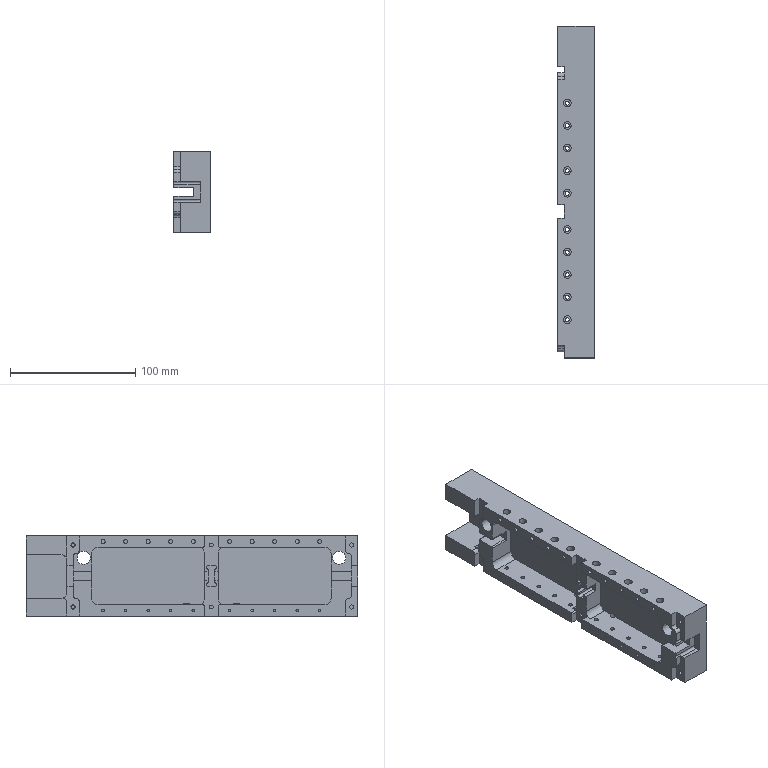CAM job | NX | 3+2 milling, drilling | part box 29 x 265 x 64 mm | stock box 35 x 270 x 65 mm
Tools:
number,name,description,diameter,corner_radius,flute_length,length,flutes
4,D4,平底铣刀-粗,4.0,0.0,25.0,75.0,2
6,D6,平底铣刀-粗,6.0,0.0,25.0,75.0,2
9,D10,平底铣刀-粗,10.0,0.0,35.0,75.0,2
19,D2-J,平底铣刀-精,2.0,0.0,50.0,75.0,2
11,D4-J,平底铣刀-精,4.0,0.0,50.0,75.0,2
7,D6-J,平底铣刀-精,6.0,0.0,25.0,75.0,2
10,D10-J,平底铣刀-精,10.0,0.0,35.0,75.0,2
1,D80R0.8飞刀,圆鼻刀-粗,80.0,0.8,50.0,75.0,2
1,D80R0.8飞刀-J,圆鼻刀-精,80.0,0.8,50.0,75.0,2
2,D6倒角刀,倒角刀,6.0,0.0,3.0,25.0,2
23,M2.5X0.45,丝锥,2.05,0.0,35.0,50.0,2
21,M4X0.7,丝锥,3.3,0.0,35.0,50.0,2
18,M6X1.0,丝锥,5.0,0.0,35.0,50.0,2
17,ZT2.1,钻头,2.1,0.0,35.0,50.0,2
13,ZT3.3,钻头,3.3,0.0,35.0,50.0,2
15,ZT5,钻头,5.0,0.0,35.0,50.0,2
18,ZT10.5,钻头,10.5,0.0,35.0,50.0,2
13,钻头3.3,Twist Drill 3.3 mm,3.3,0.0,35.0,35.008,2
17,ZT2.9,Drilling Tool,2.9,0.0,35.0,50.0,2
17,ZT5.9,Drilling Tool,5.9,0.0,35.0,50.0,2
Operations:
program,operation,operation_type,tool,method,geometry_group,spindle_rpm,surface_speed,feed_per_tooth,feed_cut,feed_plunge,cut_length_mm,path_length_mm,cut_time_min,machine_time_min
D,打点-深0.8_3,Operation,D6倒角刀,NONE,W-D,8000.0,150.796,0.0312,500.0,90.0,18.0,258.239,0.036,0.06
D,通孔-精孔6.0预钻,Operation,ZT5.9,NONE,W-D,2500.0,46.339,0.05,250.0,90.0,147.032,516.303,0.5881,0.6251
D,铣倒角_4,PlanarMilling,D6倒角刀,METHOD,W-D,8000.0,150.796,0.0312,500.0,100.0,212.261,807.104,0.4245,0.484
D,铣孔精光D4-J_1,CylinderMilling,D4-J,精光步距切深关,W-D,8000.0,100.531,0.0125,200.0,100.0,717.344,1153.344,3.587,3.63
D,铣孔精光D4-J_2,CylinderMilling,D4-J,精光步距切深关,W-D,8000.0,100.531,0.0125,200.0,100.0,717.344,1117.344,3.587,3.627
C,打点-深0.8_2,Operation,D6倒角刀,NONE,W-C,8000.0,150.796,0.0312,500.0,90.0,21.6,297.447,0.0432,0.0708
C,通孔-精孔3.0预钻,Operation,ZT2.9,NONE,W-C,3200.0,29.154,0.0312,200.0,90.0,138.372,498.982,0.6919,0.7279
C,盲平孔-M6螺纹底孔,Operation,ZT5,NONE,W-C,2800.0,43.982,0.0536,300.0,90.0,22.0,125.013,0.0733,0.0836
C,钻倒角_1,Operation,D6倒角刀,METHOD,W-C,8000.0,150.796,0.0312,500.0,0.0,48.5,339.141,0.097,0.1261
C,铣倒角_3,PlanarMilling,D6倒角刀,METHOD,W-C,8000.0,150.796,0.0312,500.0,100.0,38.882,163.579,0.0778,0.0902
C,盲平孔-攻牙M6,Operation,M6X1.0,METHOD,W-C,500.0,7.854,0.001,1.0,90.0,18.0,117.013,18.0,18.01
C,铣孔精光D2_1,CylinderMilling,D2-J,精光步距切深关,W-C,8000.0,50.266,0.0125,200.0,100.0,761.969,1460.969,3.81,3.88
B,底壁铣飞面一刀开粗_COPY,VolumeBased25DMillingOperation,D80R0.8飞刀,分层开粗-切深K-步距G,W-B,2800.0,703.696,0.5357,3000.0,100.0,4478.328,8826.038,1.493,1.927
B,底壁铣飞面一刀精光_COPY,VolumeBased25DMillingOperation,D80R0.8飞刀-J,侧刃精光-切深K-步距G,W-B,4000.0,1005.28,0.125,1000.0,100.0,372.998,408.998,0.373,0.3766
B,铣倒角_2,PlanarMilling,D6倒角刀,METHOD,W-B,8000.0,150.796,0.075,1200.0,100.0,64.732,355.932,0.0539,0.0831
B,C0.3封闭铣廓倒角6X45L_COPY,PlanarMilling,D6倒角刀,爬面_倒角-切深0-步距G,W-B,7000.0,131.0,0.1071,1500.0,100.0,675.116,711.116,0.4501,0.4537
A,顶面,FaceMilling,D80R0.8飞刀,侧刃精光-切深K-步距G,W-A,5000.0,1256.637,0.1,1000.0,100.0,752.0,788.0,0.752,0.7556
A,打点,Operation,D6倒角刀,METHOD,W-A,3000.0,56.0,0.0333,200.0,0.0,20.4,380.13,0.102,0.138
A,预钻孔3,Operation,ZT2.1,METHOD,W-A,3800.0,25.07,0.0132,100.0,0.0,176.0,691.33,1.76,1.812
A,外形粗_2,VolumeBased25DMillingOperation,D10,METHOD,W-A,8000.0,251.327,0.3125,5000.0,80.0,26913.243,26981.243,5.383,5.389
A,底壁粗_1,VolumeBased25DMillingOperation,D10,METHOD,W-A,8000.0,251.327,0.2188,3500.0,100.0,48611.69,51477.834,13.889,14.176
A,台阶粗_2,CavityMilling,D10,METHOD,W-A,8000.0,251.327,0.2188,3500.0,100.0,9887.706,10810.806,2.825,2.917
A,底壁铣分层开粗-中_COPY_1,VolumeBased25DMillingOperation,D6,分层开粗-切深K-步距G,W-A,8000.0,150.792,0.1875,3000.0,100.0,3705.616,3734.706,1.235,1.238
A,底壁粗_4,VolumeBased25DMillingOperation,D6,METHOD,W-A,6000.0,113.0,0.2083,3500.0,100.0,2467.016,2764.35,0.7049,0.7346
A,底壁粗_5,VolumeBased25DMillingOperation,D6,METHOD,W-A,6000.0,113.0,0.2083,3500.0,100.0,1740.863,2047.541,0.4974,0.5281
A,底壁粗_6,VolumeBased25DMillingOperation,D6,METHOD,W-A,6000.0,113.0,0.2083,3500.0,100.0,1623.863,1930.541,0.464,0.4946
A,底壁铣分层开粗-中_COPY_2,VolumeBased25DMillingOperation,D6,分层开粗-切深K-步距G,W-A,8000.0,150.792,0.1875,3000.0,100.0,996.16,1047.792,0.3321,0.3372
A,底壁铣螺旋开粗-中_COPY,VolumeBased25DMillingOperation,D4,分层开粗-切深K-步距G,W-A,8000.0,100.528,0.125,2000.0,100.0,2141.334,2205.233,1.071,1.077
A,底壁铣分层开粗-中_COPY,VolumeBased25DMillingOperation,D4,分层开粗-切深K-步距G,W-A,8000.0,150.796,0.125,2000.0,100.0,3586.793,3722.164,1.793,1.807
A,底壁粗_3,VolumeBased25DMillingOperation,D4,METHOD,W-A,6000.0,75.398,0.1,1200.0,100.0,6098.453,7348.655,5.082,5.207
A,打点0.8,Operation,D6倒角刀,METHOD,W-A,8000.0,150.796,0.0312,500.0,0.0,3.6,252.202,0.0072,0.0321
A,打点-深1,Operation,D6倒角刀,NONE,W-A,8000.0,150.796,0.0312,500.0,90.0,46.8,670.674,0.0936,0.156
A,打点-深0.8,Operation,D6倒角刀,NONE,W-A,8000.0,150.796,0.0312,500.0,90.0,46.8,670.674,0.0936,0.156
A,盲平孔-M2.5螺纹底孔,Operation,ZT2.1,NONE,W-A,3000.0,18.85,0.0333,200.0,90.0,110.0,442.239,0.55,0.5832
A,盲平孔-M4螺纹底孔,Operation,ZT3.3,NONE,W-A,3000.0,30.159,0.0417,250.0,90.0,26.0,152.51,0.104,0.1167
A,盲锥孔-M4螺纹底孔_2,Operation,钻头3.3,NONE,W-A,3000.0,31.102,0.0417,250.0,90.0,143.263,672.634,0.5731,0.626
A,钻倒角_5,Operation,D6倒角刀,METHOD,W-A,8000.0,150.796,0.0312,500.0,0.0,45.0,332.141,0.09,0.1187
A,钻倒角_6,Operation,D6倒角刀,METHOD,W-A,8000.0,150.796,0.0312,500.0,0.0,10.3,123.191,0.0206,0.0319
A,钻倒角_7,Operation,D6倒角刀,METHOD,W-A,8000.0,150.796,0.0312,500.0,0.0,72.8,560.096,0.1456,0.1943
A,盲平孔-攻牙M2.5,Operation,M2.5X0.45,METHOD,W-A,1000.0,6.44,0.0002,0.45,90.0,80.0,382.239,177.778,177.808
A,盲平孔-攻牙M4,Operation,M4X0.7,METHOD,W-A,800.0,8.294,0.0004,0.7,90.0,145.349,838.794,207.641,207.71
A,盲平孔-攻牙M4_COPY,Operation,M4X0.7,METHOD,W-A,800.0,8.294,0.0004,0.7,90.0,20.0,140.51,28.571,28.584
A,通孔-10-12.5,Operation,ZT10.5,NONE,W-A,1500.0,49.48,0.1,300.0,90.0,70.309,385.62,0.2344,0.2659
A,底精_8,VolumeBased25DMillingOperation,D4-J,METHOD,W-A,6000.0,113.0,0.2083,1200.0,100.0,79.4,483.901,0.0662,0.1066
A,底精_3,VolumeBased25DMillingOperation,D4-J,METHOD,W-A,6000.0,113.0,0.2083,1200.0,100.0,99.299,148.299,0.0827,0.0876
A,底精_4,VolumeBased25DMillingOperation,D4-J,METHOD,W-A,6000.0,113.0,0.2083,1200.0,100.0,99.747,148.747,0.0831,0.088
A,底精_5,VolumeBased25DMillingOperation,D4-J,METHOD,W-A,6000.0,113.0,0.2083,1200.0,100.0,210.272,358.506,0.1752,0.19
A,底精_1,VolumeBased25DMillingOperation,D6-J,METHOD,W-A,6000.0,113.0,0.2083,1200.0,100.0,2091.524,2311.95,1.743,1.765
A,底精_2,VolumeBased25DMillingOperation,D6-J,METHOD,W-A,6000.0,113.0,0.2083,1200.0,100.0,287.641,379.641,0.2397,0.2489
A,底壁铣精光底面-中_COPY,VolumeBased25DMillingOperation,D6-J,精光步距切深关,W-A,8000.0,150.792,0.0625,1000.0,100.0,314.258,342.058,0.3143,0.317
A,清角D2,ZLevelMilling,D2-J,METHOD,W-A,7000.0,43.982,0.1429,2000.0,80.0,3668.569,3934.997,1.836,1.863
A,清角D2_COPY,ZLevelMilling,D2-J,METHOD,W-A,7000.0,43.982,0.1429,2000.0,80.0,3524.581,4008.387,1.764,1.812
A,仅选体,SurfaceContour,D6倒角刀,METHOD,W-A,8000.0,150.796,0.1875,3000.0,100.0,2226.895,4753.559,0.7423,0.995
A,铣倒角_1,PlanarMilling,D6倒角刀,METHOD,W-A,8000.0,150.796,0.05,800.0,100.0,78.026,364.05,0.0975,0.1261
A,底壁铣精光侧面-中-选底面_COPY_1,VolumeBased25DMillingOperation,D6-J,侧刃精光-切深K-步距G,W-A,8000.0,150.792,0.0625,1000.0,100.0,92.277,142.315,0.0923,0.0973
A,底壁铣精光侧面-中-选底面_COPY,VolumeBased25DMillingOperation,D6-J,侧刃精光-切深K-步距G,W-A,8000.0,150.792,0.0625,1000.0,100.0,109.774,175.374,0.1098,0.1163
A,底侧精_8,VolumeBased25DMillingOperation,D6-J,METHOD,W-A,6000.0,113.0,0.2083,1200.0,100.0,127.299,411.269,0.1061,0.1345
A,底侧精_9,VolumeBased25DMillingOperation,D6-J,METHOD,W-A,6000.0,113.0,0.2083,1200.0,100.0,120.499,261.984,0.1004,0.1146
A,底侧精_3,VolumeBased25DMillingOperation,D6-J,METHOD,W-A,6000.0,113.0,0.2083,1200.0,100.0,1496.448,2011.908,1.247,1.299
A,底侧精_4,VolumeBased25DMillingOperation,D6-J,METHOD,W-A,6000.0,113.0,0.2083,1200.0,100.0,385.099,754.724,0.3209,0.3579
A,底侧精_7,VolumeBased25DMillingOperation,D4-J,METHOD,W-A,6000.0,75.398,0.05,600.0,100.0,69.619,178.326,0.116,0.1269
A,底侧精_5,VolumeBased25DMillingOperation,D4-J,METHOD,W-A,6000.0,113.0,0.2083,1200.0,100.0,67.94,116.93,0.0566,0.0615
A,底侧精_6,VolumeBased25DMillingOperation,D4-J,METHOD,W-A,6000.0,113.0,0.2083,1200.0,100.0,93.905,142.895,0.0783,0.0832
A,底侧精_10,VolumeBased25DMillingOperation,D4-J,METHOD,W-A,6000.0,113.0,0.05,600.0,100.0,260.864,1219.784,0.4348,0.5307
A,底侧精_11,VolumeBased25DMillingOperation,D4-J,METHOD,W-A,6000.0,113.0,0.2083,1200.0,100.0,59.691,206.776,0.0497,0.0645
A,外形半精_2,VolumeBased25DMillingOperation,D10-J,METHOD,W-A,8000.0,251.327,0.0625,1000.0,100.0,1388.748,1557.763,1.389,1.406